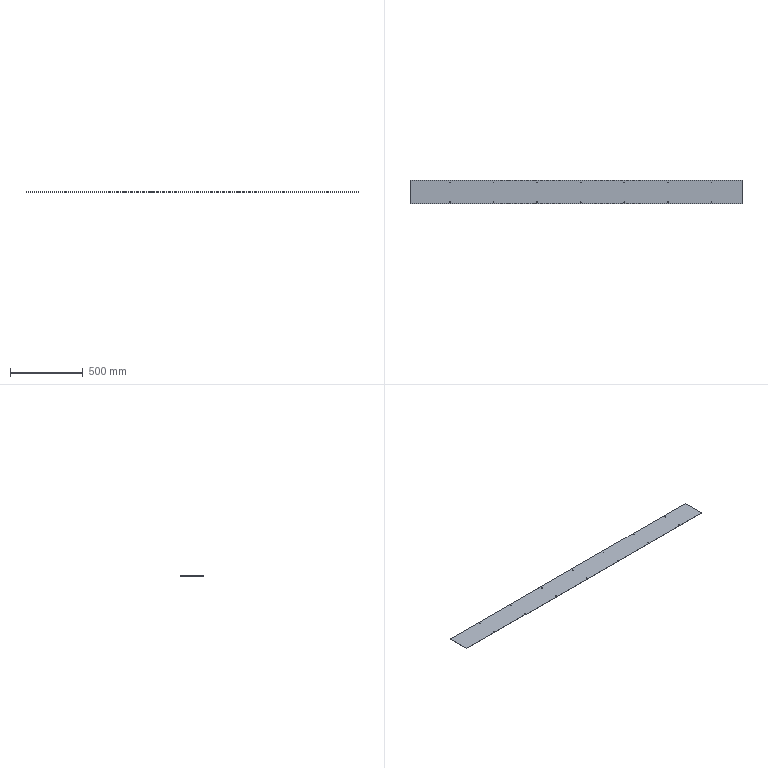Part | STEP file | SX-S20 | 1 solid | 34 faces | box 2285 x 159.5 x 1.2 mm | volume 436964 mm3 | cylinder 28 | plane 6 | commonest cylinder face diameters 5.4 x28